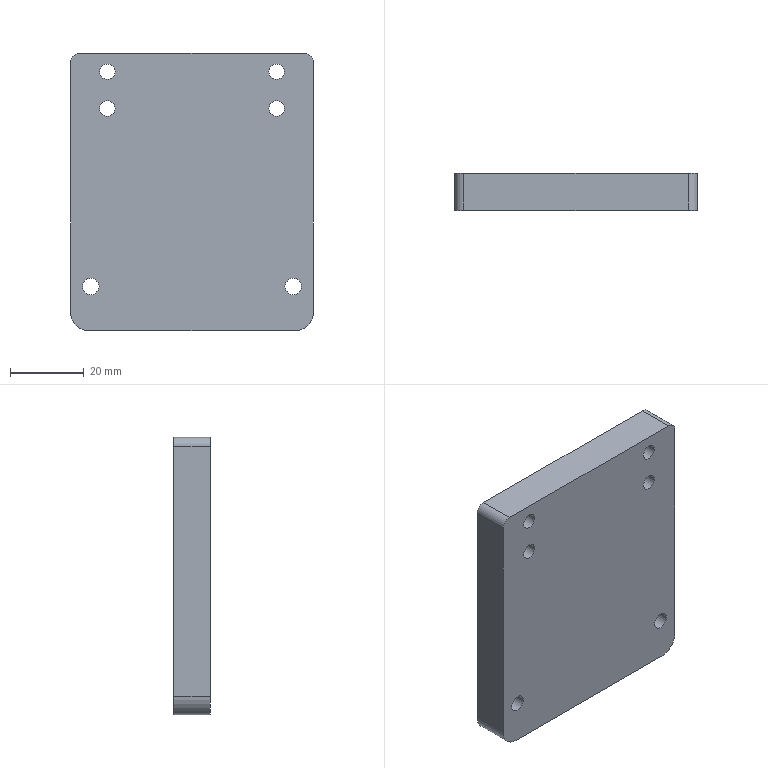Part | SolidWorks | features BaseBody 1 | 1 solid | 40 faces | box 66 x 10 x 75.35 mm | volume 47694 mm3 | cylinder 28 | plane 12 | commonest cylinder face diameters 8 x12 4.2 x8 4.5 x4 5 x2 10 x2
STEP:
#1=CARTESIAN_POINT('',(-707.631,758.297,277.132));
#2=VERTEX_POINT('',#1);
#3=CARTESIAN_POINT('',(-702.631,758.297,282.132));
#4=VERTEX_POINT('',#3);
#5=CARTESIAN_POINT('',(-707.631,758.297,282.132));
#6=DIRECTION('',(0.,-1.,0.));
#7=DIRECTION('',(0.,0.,-1.));
#8=AXIS2_PLACEMENT_3D('',#5,#6,#7);
#9=CIRCLE('',#8,5.);
#10=EDGE_CURVE('',#2,#4,#9,.T.);
#11=ORIENTED_EDGE('',*,*,#10,.F.);
#12=CARTESIAN_POINT('',(-763.631,758.297,277.132));
#13=VERTEX_POINT('',#12);
#14=CARTESIAN_POINT('',(-763.631,758.297,277.132));
#15=DIRECTION('',(1.,0.,0.));
#16=VECTOR('',#15,1000.);
#17=LINE('',#14,#16);
#18=EDGE_CURVE('',#13,#2,#17,.T.);
#19=ORIENTED_EDGE('',*,*,#18,.F.);
#20=CARTESIAN_POINT('',(-768.631,758.297,282.132));
#21=VERTEX_POINT('',#20);
#22=CARTESIAN_POINT('',(-763.631,758.297,282.132));
#23=DIRECTION('',(0.,-1.,0.));
#24=DIRECTION('',(-1.,0.,0.));
#25=AXIS2_PLACEMENT_3D('',#22,#23,#24);
#26=CIRCLE('',#25,5.);
#27=EDGE_CURVE('',#21,#13,#26,.T.);
#28=ORIENTED_EDGE('',*,*,#27,.F.);
#29=CARTESIAN_POINT('',(-768.631,758.297,349.982));
#30=VERTEX_POINT('',#29);
#31=CARTESIAN_POINT('',(-768.631,758.297,349.982));
#32=DIRECTION('',(0.,0.,-1.));
#33=VECTOR('',#32,1000.);
#34=LINE('',#31,#33);
#35=EDGE_CURVE('',#30,#21,#34,.T.);
#36=ORIENTED_EDGE('',*,*,#35,.F.);
#37=CARTESIAN_POINT('',(-766.131,758.297,352.482));
#38=VERTEX_POINT('',#37);
#39=CARTESIAN_POINT('',(-766.131,758.297,349.982));
#40=DIRECTION('',(0.,-1.,0.));
#41=DIRECTION('',(0.,0.,1.));
#42=AXIS2_PLACEMENT_3D('',#39,#40,#41);
#43=CIRCLE('',#42,2.5);
#44=EDGE_CURVE('',#38,#30,#43,.T.);
#45=ORIENTED_EDGE('',*,*,#44,.F.);
#46=CARTESIAN_POINT('',(-705.131,758.297,352.482));
#47=VERTEX_POINT('',#46);
#48=CARTESIAN_POINT('',(-705.131,758.297,352.482));
#49=DIRECTION('',(-1.,0.,0.));
#50=VECTOR('',#49,1000.);
#51=LINE('',#48,#50);
#52=EDGE_CURVE('',#47,#38,#51,.T.);
#53=ORIENTED_EDGE('',*,*,#52,.F.);
#54=CARTESIAN_POINT('',(-702.631,758.297,349.982));
#55=VERTEX_POINT('',#54);
#56=CARTESIAN_POINT('',(-705.131,758.297,349.982));
#57=DIRECTION('',(0.,-1.,0.));
#58=DIRECTION('',(1.,0.,0.));
#59=AXIS2_PLACEMENT_3D('',#56,#57,#58);
#60=CIRCLE('',#59,2.5);
#61=EDGE_CURVE('',#55,#47,#60,.T.);
#62=ORIENTED_EDGE('',*,*,#61,.F.);
#63=CARTESIAN_POINT('',(-702.631,758.297,282.132));
#64=DIRECTION('',(0.,0.,1.));
#65=VECTOR('',#64,1000.);
#66=LINE('',#63,#65);
#67=EDGE_CURVE('',#4,#55,#66,.T.);
#68=ORIENTED_EDGE('',*,*,#67,.F.);
#69=EDGE_LOOP('',(#11,#19,#28,#36,#45,#53,#62,#68));
#70=FACE_OUTER_BOUND('',#69,.T.);
#71=CARTESIAN_POINT('',(-712.131,758.297,289.132));
#72=VERTEX_POINT('',#71);
#73=CARTESIAN_POINT('',(-704.131,758.297,289.132));
#74=VERTEX_POINT('',#73);
#75=CARTESIAN_POINT('',(-708.131,758.297,289.132));
#76=DIRECTION('',(0.,1.,0.));
#77=DIRECTION('',(-1.,0.,0.));
#78=AXIS2_PLACEMENT_3D('',#75,#76,#77);
#79=CIRCLE('',#78,4.);
#80=EDGE_CURVE('',#72,#74,#79,.T.);
#81=ORIENTED_EDGE('',*,*,#80,.F.);
#82=CARTESIAN_POINT('',(-708.131,758.297,289.132));
#83=DIRECTION('',(0.,1.,0.));
#84=DIRECTION('',(1.,0.,0.));
#85=AXIS2_PLACEMENT_3D('',#82,#83,#84);
#86=CIRCLE('',#85,4.);
#87=EDGE_CURVE('',#74,#72,#86,.T.);
#88=ORIENTED_EDGE('',*,*,#87,.F.);
#89=EDGE_LOOP('',(#81,#88));
#90=FACE_BOUND('',#89,.T.);
#91=CARTESIAN_POINT('',(-716.631,758.297,347.482));
#92=VERTEX_POINT('',#91);
#93=CARTESIAN_POINT('',(-708.631,758.297,347.482));
#94=VERTEX_POINT('',#93);
#95=CARTESIAN_POINT('',(-712.631,758.297,347.482));
#96=DIRECTION('',(0.,1.,0.));
#97=DIRECTION('',(-1.,0.,0.));
#98=AXIS2_PLACEMENT_3D('',#95,#96,#97);
#99=CIRCLE('',#98,4.);
#100=EDGE_CURVE('',#92,#94,#99,.T.);
#101=ORIENTED_EDGE('',*,*,#100,.F.);
#102=CARTESIAN_POINT('',(-712.631,758.297,347.482));
#103=DIRECTION('',(0.,1.,0.));
#104=DIRECTION('',(1.,0.,0.));
#105=AXIS2_PLACEMENT_3D('',#102,#103,#104);
#106=CIRCLE('',#105,4.);
#107=EDGE_CURVE('',#94,#92,#106,.T.);
#108=ORIENTED_EDGE('',*,*,#107,.F.);
#109=EDGE_LOOP('',(#101,#108));
#110=FACE_BOUND('',#109,.T.);
#111=CARTESIAN_POINT('',(-762.631,758.297,347.482));
#112=VERTEX_POINT('',#111);
#113=CARTESIAN_POINT('',(-754.631,758.297,347.482));
#114=VERTEX_POINT('',#113);
#115=CARTESIAN_POINT('',(-758.631,758.297,347.482));
#116=DIRECTION('',(0.,1.,0.));
#117=DIRECTION('',(-1.,0.,0.));
#118=AXIS2_PLACEMENT_3D('',#115,#116,#117);
#119=CIRCLE('',#118,4.);
#120=EDGE_CURVE('',#112,#114,#119,.T.);
#121=ORIENTED_EDGE('',*,*,#120,.F.);
#122=CARTESIAN_POINT('',(-758.631,758.297,347.482));
#123=DIRECTION('',(0.,1.,0.));
#124=DIRECTION('',(1.,0.,0.));
#125=AXIS2_PLACEMENT_3D('',#122,#123,#124);
#126=CIRCLE('',#125,4.);
#127=EDGE_CURVE('',#114,#112,#126,.T.);
#128=ORIENTED_EDGE('',*,*,#127,.F.);
#129=EDGE_LOOP('',(#121,#128));
#130=FACE_BOUND('',#129,.T.);
#131=CARTESIAN_POINT('',(-762.631,758.297,337.482));
#132=VERTEX_POINT('',#131);
#133=CARTESIAN_POINT('',(-754.631,758.297,337.482));
#134=VERTEX_POINT('',#133);
#135=CARTESIAN_POINT('',(-758.631,758.297,337.482));
#136=DIRECTION('',(0.,1.,0.));
#137=DIRECTION('',(-1.,0.,0.));
#138=AXIS2_PLACEMENT_3D('',#135,#136,#137);
#139=CIRCLE('',#138,4.);
#140=EDGE_CURVE('',#132,#134,#139,.T.);
#141=ORIENTED_EDGE('',*,*,#140,.F.);
#142=CARTESIAN_POINT('',(-758.631,758.297,337.482));
#143=DIRECTION('',(0.,1.,0.));
#144=DIRECTION('',(1.,0.,0.));
#145=AXIS2_PLACEMENT_3D('',#142,#143,#144);
#146=CIRCLE('',#145,4.);
#147=EDGE_CURVE('',#134,#132,#146,.T.);
#148=ORIENTED_EDGE('',*,*,#147,.F.);
#149=EDGE_LOOP('',(#141,#148));
#150=FACE_BOUND('',#149,.T.);
#151=CARTESIAN_POINT('',(-716.631,758.297,337.482));
#152=VERTEX_POINT('',#151);
#153=CARTESIAN_POINT('',(-708.631,758.297,337.482));
#154=VERTEX_POINT('',#153);
#155=CARTESIAN_POINT('',(-712.631,758.297,337.482));
#156=DIRECTION('',(0.,1.,0.));
#157=DIRECTION('',(-1.,0.,0.));
#158=AXIS2_PLACEMENT_3D('',#155,#156,#157);
#159=CIRCLE('',#158,4.);
#160=EDGE_CURVE('',#152,#154,#159,.T.);
#161=ORIENTED_EDGE('',*,*,#160,.F.);
#162=CARTESIAN_POINT('',(-712.631,758.297,337.482));
#163=DIRECTION('',(0.,1.,0.));
#164=DIRECTION('',(1.,0.,0.));
#165=AXIS2_PLACEMENT_3D('',#162,#163,#164);
#166=CIRCLE('',#165,4.);
#167=EDGE_CURVE('',#154,#152,#166,.T.);
#168=ORIENTED_EDGE('',*,*,#167,.F.);
#169=EDGE_LOOP('',(#161,#168));
#170=FACE_BOUND('',#169,.T.);
#171=CARTESIAN_POINT('',(-767.131,758.297,289.132));
#172=VERTEX_POINT('',#171);
#173=CARTESIAN_POINT('',(-759.131,758.297,289.132));
#174=VERTEX_POINT('',#173);
#175=CARTESIAN_POINT('',(-763.131,758.297,289.132));
#176=DIRECTION('',(0.,1.,0.));
#177=DIRECTION('',(-1.,0.,0.));
#178=AXIS2_PLACEMENT_3D('',#175,#176,#177);
#179=CIRCLE('',#178,4.);
#180=EDGE_CURVE('',#172,#174,#179,.T.);
#181=ORIENTED_EDGE('',*,*,#180,.F.);
#182=CARTESIAN_POINT('',(-763.131,758.297,289.132));
#183=DIRECTION('',(0.,1.,0.));
#184=DIRECTION('',(1.,0.,0.));
#185=AXIS2_PLACEMENT_3D('',#182,#183,#184);
#186=CIRCLE('',#185,4.);
#187=EDGE_CURVE('',#174,#172,#186,.T.);
#188=ORIENTED_EDGE('',*,*,#187,.F.);
#189=EDGE_LOOP('',(#181,#188));
#190=FACE_BOUND('',#189,.T.);
#191=CARTESIAN_POINT('',(-735.631,758.297,320.932));
#192=DIRECTION('',(0.,1.,0.));
#193=DIRECTION('',(1.,0.,0.));
#194=AXIS2_PLACEMENT_3D('',#191,#192,#193);
#195=PLANE('',#194);
#196=ADVANCED_FACE('',(#70,#90,#110,#130,#150,#170,#190),#195,.T.);
#197=CARTESIAN_POINT('',(-702.631,748.297,282.132));
#198=VERTEX_POINT('',#197);
#199=CARTESIAN_POINT('',(-702.631,748.297,282.132));
#200=DIRECTION('',(0.,1.,0.));
#201=VECTOR('',#200,1000.);
#202=LINE('',#199,#201);
#203=EDGE_CURVE('',#198,#4,#202,.T.);
#204=ORIENTED_EDGE('',*,*,#203,.T.);
#205=ORIENTED_EDGE('',*,*,#67,.T.);
#206=CARTESIAN_POINT('',(-702.631,748.297,349.982));
#207=VERTEX_POINT('',#206);
#208=CARTESIAN_POINT('',(-702.631,758.297,349.982));
#209=DIRECTION('',(0.,-1.,0.));
#210=VECTOR('',#209,1000.);
#211=LINE('',#208,#210);
#212=EDGE_CURVE('',#55,#207,#211,.T.);
#213=ORIENTED_EDGE('',*,*,#212,.T.);
#214=CARTESIAN_POINT('',(-702.631,748.297,349.982));
#215=DIRECTION('',(0.,0.,-1.));
#216=VECTOR('',#215,1000.);
#217=LINE('',#214,#216);
#218=EDGE_CURVE('',#207,#198,#217,.T.);
#219=ORIENTED_EDGE('',*,*,#218,.T.);
#220=EDGE_LOOP('',(#204,#205,#213,#219));
#221=FACE_OUTER_BOUND('',#220,.T.);
#222=CARTESIAN_POINT('',(-702.631,758.297,277.132));
#223=DIRECTION('',(-1.,0.,0.));
#224=DIRECTION('',(0.,1.,0.));
#225=AXIS2_PLACEMENT_3D('',#222,#223,#224);
#226=PLANE('',#225);
#227=ADVANCED_FACE('',(#221),#226,.F.);
#228=CARTESIAN_POINT('',(-768.631,748.297,349.982));
#229=VERTEX_POINT('',#228);
#230=CARTESIAN_POINT('',(-766.131,748.297,352.482));
#231=VERTEX_POINT('',#230);
#232=CARTESIAN_POINT('',(-766.131,748.297,349.982));
#233=DIRECTION('',(0.,1.,0.));
#234=DIRECTION('',(-1.,0.,0.));
#235=AXIS2_PLACEMENT_3D('',#232,#233,#234);
#236=CIRCLE('',#235,2.5);
#237=EDGE_CURVE('',#229,#231,#236,.T.);
#238=ORIENTED_EDGE('',*,*,#237,.F.);
#239=CARTESIAN_POINT('',(-768.631,748.297,282.132));
#240=VERTEX_POINT('',#239);
#241=CARTESIAN_POINT('',(-768.631,748.297,282.132));
#242=DIRECTION('',(0.,0.,1.));
#243=VECTOR('',#242,1000.);
#244=LINE('',#241,#243);
#245=EDGE_CURVE('',#240,#229,#244,.T.);
#246=ORIENTED_EDGE('',*,*,#245,.F.);
#247=CARTESIAN_POINT('',(-763.631,748.297,277.132));
#248=VERTEX_POINT('',#247);
#249=CARTESIAN_POINT('',(-763.631,748.297,282.132));
#250=DIRECTION('',(0.,1.,0.));
#251=DIRECTION('',(0.,0.,-1.));
#252=AXIS2_PLACEMENT_3D('',#249,#250,#251);
#253=CIRCLE('',#252,5.);
#254=EDGE_CURVE('',#248,#240,#253,.T.);
#255=ORIENTED_EDGE('',*,*,#254,.F.);
#256=CARTESIAN_POINT('',(-707.631,748.297,277.132));
#257=VERTEX_POINT('',#256);
#258=CARTESIAN_POINT('',(-707.631,748.297,277.132));
#259=DIRECTION('',(-1.,0.,0.));
#260=VECTOR('',#259,1000.);
#261=LINE('',#258,#260);
#262=EDGE_CURVE('',#257,#248,#261,.T.);
#263=ORIENTED_EDGE('',*,*,#262,.F.);
#264=CARTESIAN_POINT('',(-707.631,748.297,282.132));
#265=DIRECTION('',(0.,1.,0.));
#266=DIRECTION('',(1.,0.,0.));
#267=AXIS2_PLACEMENT_3D('',#264,#265,#266);
#268=CIRCLE('',#267,5.);
#269=EDGE_CURVE('',#198,#257,#268,.T.);
#270=ORIENTED_EDGE('',*,*,#269,.F.);
#271=ORIENTED_EDGE('',*,*,#218,.F.);
#272=CARTESIAN_POINT('',(-705.131,748.297,352.482));
#273=VERTEX_POINT('',#272);
#274=CARTESIAN_POINT('',(-705.131,748.297,349.982));
#275=DIRECTION('',(0.,1.,0.));
#276=DIRECTION('',(0.,0.,1.));
#277=AXIS2_PLACEMENT_3D('',#274,#275,#276);
#278=CIRCLE('',#277,2.5);
#279=EDGE_CURVE('',#273,#207,#278,.T.);
#280=ORIENTED_EDGE('',*,*,#279,.F.);
#281=CARTESIAN_POINT('',(-766.131,748.297,352.482));
#282=DIRECTION('',(1.,0.,0.));
#283=VECTOR('',#282,1000.);
#284=LINE('',#281,#283);
#285=EDGE_CURVE('',#231,#273,#284,.T.);
#286=ORIENTED_EDGE('',*,*,#285,.F.);
#287=EDGE_LOOP('',(#238,#246,#255,#263,#270,#271,#280,#286));
#288=FACE_OUTER_BOUND('',#287,.T.);
#289=CARTESIAN_POINT('',(-705.881,748.297,289.132));
#290=VERTEX_POINT('',#289);
#291=CARTESIAN_POINT('',(-710.381,748.297,289.132));
#292=VERTEX_POINT('',#291);
#293=CARTESIAN_POINT('',(-708.131,748.297,289.132));
#294=DIRECTION('',(0.,-1.,0.));
#295=DIRECTION('',(1.,0.,0.));
#296=AXIS2_PLACEMENT_3D('',#293,#294,#295);
#297=CIRCLE('',#296,2.25);
#298=EDGE_CURVE('',#290,#292,#297,.T.);
#299=ORIENTED_EDGE('',*,*,#298,.F.);
#300=CARTESIAN_POINT('',(-708.131,748.297,289.132));
#301=DIRECTION('',(0.,-1.,0.));
#302=DIRECTION('',(-1.,0.,0.));
#303=AXIS2_PLACEMENT_3D('',#300,#301,#302);
#304=CIRCLE('',#303,2.25);
#305=EDGE_CURVE('',#292,#290,#304,.T.);
#306=ORIENTED_EDGE('',*,*,#305,.F.);
#307=EDGE_LOOP('',(#299,#306));
#308=FACE_BOUND('',#307,.T.);
#309=CARTESIAN_POINT('',(-710.531,748.297,347.482));
#310=VERTEX_POINT('',#309);
#311=CARTESIAN_POINT('',(-714.731,748.297,347.482));
#312=VERTEX_POINT('',#311);
#313=CARTESIAN_POINT('',(-712.631,748.297,347.482));
#314=DIRECTION('',(0.,-1.,0.));
#315=DIRECTION('',(1.,0.,0.));
#316=AXIS2_PLACEMENT_3D('',#313,#314,#315);
#317=CIRCLE('',#316,2.1);
#318=EDGE_CURVE('',#310,#312,#317,.T.);
#319=ORIENTED_EDGE('',*,*,#318,.F.);
#320=CARTESIAN_POINT('',(-712.631,748.297,347.482));
#321=DIRECTION('',(0.,-1.,0.));
#322=DIRECTION('',(-1.,0.,0.));
#323=AXIS2_PLACEMENT_3D('',#320,#321,#322);
#324=CIRCLE('',#323,2.1);
#325=EDGE_CURVE('',#312,#310,#324,.T.);
#326=ORIENTED_EDGE('',*,*,#325,.F.);
#327=EDGE_LOOP('',(#319,#326));
#328=FACE_BOUND('',#327,.T.);
#329=CARTESIAN_POINT('',(-756.531,748.297,347.482));
#330=VERTEX_POINT('',#329);
#331=CARTESIAN_POINT('',(-760.731,748.297,347.482));
#332=VERTEX_POINT('',#331);
#333=CARTESIAN_POINT('',(-758.631,748.297,347.482));
#334=DIRECTION('',(0.,-1.,0.));
#335=DIRECTION('',(1.,0.,0.));
#336=AXIS2_PLACEMENT_3D('',#333,#334,#335);
#337=CIRCLE('',#336,2.1);
#338=EDGE_CURVE('',#330,#332,#337,.T.);
#339=ORIENTED_EDGE('',*,*,#338,.F.);
#340=CARTESIAN_POINT('',(-758.631,748.297,347.482));
#341=DIRECTION('',(0.,-1.,0.));
#342=DIRECTION('',(-1.,0.,0.));
#343=AXIS2_PLACEMENT_3D('',#340,#341,#342);
#344=CIRCLE('',#343,2.1);
#345=EDGE_CURVE('',#332,#330,#344,.T.);
#346=ORIENTED_EDGE('',*,*,#345,.F.);
#347=EDGE_LOOP('',(#339,#346));
#348=FACE_BOUND('',#347,.T.);
#349=CARTESIAN_POINT('',(-710.531,748.297,337.482));
#350=VERTEX_POINT('',#349);
#351=CARTESIAN_POINT('',(-714.731,748.297,337.482));
#352=VERTEX_POINT('',#351);
#353=CARTESIAN_POINT('',(-712.631,748.297,337.482));
#354=DIRECTION('',(0.,-1.,0.));
#355=DIRECTION('',(1.,0.,0.));
#356=AXIS2_PLACEMENT_3D('',#353,#354,#355);
#357=CIRCLE('',#356,2.1);
#358=EDGE_CURVE('',#350,#352,#357,.T.);
#359=ORIENTED_EDGE('',*,*,#358,.F.);
#360=CARTESIAN_POINT('',(-712.631,748.297,337.482));
#361=DIRECTION('',(0.,-1.,0.));
#362=DIRECTION('',(-1.,0.,0.));
#363=AXIS2_PLACEMENT_3D('',#360,#361,#362);
#364=CIRCLE('',#363,2.1);
#365=EDGE_CURVE('',#352,#350,#364,.T.);
#366=ORIENTED_EDGE('',*,*,#365,.F.);
#367=EDGE_LOOP('',(#359,#366));
#368=FACE_BOUND('',#367,.T.);
#369=CARTESIAN_POINT('',(-756.531,748.297,337.482));
#370=VERTEX_POINT('',#369);
#371=CARTESIAN_POINT('',(-760.731,748.297,337.482));
#372=VERTEX_POINT('',#371);
#373=CARTESIAN_POINT('',(-758.631,748.297,337.482));
#374=DIRECTION('',(0.,-1.,0.));
#375=DIRECTION('',(1.,0.,0.));
#376=AXIS2_PLACEMENT_3D('',#373,#374,#375);
#377=CIRCLE('',#376,2.1);
#378=EDGE_CURVE('',#370,#372,#377,.T.);
#379=ORIENTED_EDGE('',*,*,#378,.F.);
#380=CARTESIAN_POINT('',(-758.631,748.297,337.482));
#381=DIRECTION('',(0.,-1.,0.));
#382=DIRECTION('',(-1.,0.,0.));
#383=AXIS2_PLACEMENT_3D('',#380,#381,#382);
#384=CIRCLE('',#383,2.1);
#385=EDGE_CURVE('',#372,#370,#384,.T.);
#386=ORIENTED_EDGE('',*,*,#385,.F.);
#387=EDGE_LOOP('',(#379,#386));
#388=FACE_BOUND('',#387,.T.);
#389=CARTESIAN_POINT('',(-760.881,748.297,289.132));
#390=VERTEX_POINT('',#389);
#391=CARTESIAN_POINT('',(-765.381,748.297,289.132));
#392=VERTEX_POINT('',#391);
#393=CARTESIAN_POINT('',(-763.131,748.297,289.132));
#394=DIRECTION('',(0.,-1.,0.));
#395=DIRECTION('',(1.,0.,0.));
#396=AXIS2_PLACEMENT_3D('',#393,#394,#395);
#397=CIRCLE('',#396,2.25);
#398=EDGE_CURVE('',#390,#392,#397,.T.);
#399=ORIENTED_EDGE('',*,*,#398,.F.);
#400=CARTESIAN_POINT('',(-763.131,748.297,289.132));
#401=DIRECTION('',(0.,-1.,0.));
#402=DIRECTION('',(-1.,0.,0.));
#403=AXIS2_PLACEMENT_3D('',#400,#401,#402);
#404=CIRCLE('',#403,2.25);
#405=EDGE_CURVE('',#392,#390,#404,.T.);
#406=ORIENTED_EDGE('',*,*,#405,.F.);
#407=EDGE_LOOP('',(#399,#406));
#408=FACE_BOUND('',#407,.T.);
#409=CARTESIAN_POINT('',(-735.631,748.297,320.932));
#410=DIRECTION('',(0.,1.,0.));
#411=DIRECTION('',(1.,0.,0.));
#412=AXIS2_PLACEMENT_3D('',#409,#410,#411);
#413=PLANE('',#412);
#414=ADVANCED_FACE('',(#288,#308,#328,#348,#368,#388,#408),#413,.F.);
#415=CARTESIAN_POINT('',(-766.131,758.297,352.482));
#416=DIRECTION('',(0.,-1.,0.));
#417=VECTOR('',#416,1000.);
#418=LINE('',#415,#417);
#419=EDGE_CURVE('',#38,#231,#418,.T.);
#420=ORIENTED_EDGE('',*,*,#419,.T.);
#421=ORIENTED_EDGE('',*,*,#285,.T.);
#422=CARTESIAN_POINT('',(-705.131,748.297,352.482));
#423=DIRECTION('',(0.,1.,0.));
#424=VECTOR('',#423,1000.);
#425=LINE('',#422,#424);
#426=EDGE_CURVE('',#273,#47,#425,.T.);
#427=ORIENTED_EDGE('',*,*,#426,.T.);
#428=ORIENTED_EDGE('',*,*,#52,.T.);
#429=EDGE_LOOP('',(#420,#421,#427,#428));
#430=FACE_OUTER_BOUND('',#429,.T.);
#431=CARTESIAN_POINT('',(-691.23,758.297,352.482));
#432=DIRECTION('',(0.,0.,-1.));
#433=DIRECTION('',(1.,0.,0.));
#434=AXIS2_PLACEMENT_3D('',#431,#432,#433);
#435=PLANE('',#434);
#436=ADVANCED_FACE('',(#430),#435,.F.);
#437=ORIENTED_EDGE('',*,*,#61,.T.);
#438=ORIENTED_EDGE('',*,*,#426,.F.);
#439=ORIENTED_EDGE('',*,*,#279,.T.);
#440=ORIENTED_EDGE('',*,*,#212,.F.);
#441=EDGE_LOOP('',(#437,#438,#439,#440));
#442=FACE_OUTER_BOUND('',#441,.T.);
#443=CARTESIAN_POINT('',(-705.131,771.333,349.982));
#444=DIRECTION('',(0.,-1.,0.));
#445=DIRECTION('',(-1.,0.,0.));
#446=AXIS2_PLACEMENT_3D('',#443,#444,#445);
#447=CYLINDRICAL_SURFACE('',#446,2.5);
#448=ADVANCED_FACE('',(#442),#447,.T.);
#449=ORIENTED_EDGE('',*,*,#237,.T.);
#450=ORIENTED_EDGE('',*,*,#419,.F.);
#451=ORIENTED_EDGE('',*,*,#44,.T.);
#452=CARTESIAN_POINT('',(-768.631,748.297,349.982));
#453=DIRECTION('',(0.,1.,0.));
#454=VECTOR('',#453,1000.);
#455=LINE('',#452,#454);
#456=EDGE_CURVE('',#229,#30,#455,.T.);
#457=ORIENTED_EDGE('',*,*,#456,.F.);
#458=EDGE_LOOP('',(#449,#450,#451,#457));
#459=FACE_OUTER_BOUND('',#458,.T.);
#460=CARTESIAN_POINT('',(-766.131,735.261,349.982));
#461=DIRECTION('',(0.,1.,0.));
#462=DIRECTION('',(1.,0.,0.));
#463=AXIS2_PLACEMENT_3D('',#460,#461,#462);
#464=CYLINDRICAL_SURFACE('',#463,2.5);
#465=ADVANCED_FACE('',(#459),#464,.T.);
#466=CARTESIAN_POINT('',(-768.631,758.297,282.132));
#467=DIRECTION('',(0.,-1.,0.));
#468=VECTOR('',#467,1000.);
#469=LINE('',#466,#468);
#470=EDGE_CURVE('',#21,#240,#469,.T.);
#471=ORIENTED_EDGE('',*,*,#470,.T.);
#472=ORIENTED_EDGE('',*,*,#245,.T.);
#473=ORIENTED_EDGE('',*,*,#456,.T.);
#474=ORIENTED_EDGE('',*,*,#35,.T.);
#475=EDGE_LOOP('',(#471,#472,#473,#474));
#476=FACE_OUTER_BOUND('',#475,.T.);
#477=CARTESIAN_POINT('',(-768.631,758.297,277.132));
#478=DIRECTION('',(1.,0.,0.));
#479=DIRECTION('',(0.,-1.,0.));
#480=AXIS2_PLACEMENT_3D('',#477,#478,#479);
#481=PLANE('',#480);
#482=ADVANCED_FACE('',(#476),#481,.F.);
#483=ORIENTED_EDGE('',*,*,#254,.T.);
#484=ORIENTED_EDGE('',*,*,#470,.F.);
#485=ORIENTED_EDGE('',*,*,#27,.T.);
#486=CARTESIAN_POINT('',(-763.631,748.297,277.132));
#487=DIRECTION('',(0.,1.,0.));
#488=VECTOR('',#487,1000.);
#489=LINE('',#486,#488);
#490=EDGE_CURVE('',#248,#13,#489,.T.);
#491=ORIENTED_EDGE('',*,*,#490,.F.);
#492=EDGE_LOOP('',(#483,#484,#485,#491));
#493=FACE_OUTER_BOUND('',#492,.T.);
#494=CARTESIAN_POINT('',(-763.631,758.297,282.132));
#495=DIRECTION('',(0.,-1.,0.));
#496=DIRECTION('',(-1.,0.,0.));
#497=AXIS2_PLACEMENT_3D('',#494,#495,#496);
#498=CYLINDRICAL_SURFACE('',#497,5.);
#499=ADVANCED_FACE('',(#493),#498,.T.);
#500=ORIENTED_EDGE('',*,*,#262,.T.);
#501=ORIENTED_EDGE('',*,*,#490,.T.);
#502=ORIENTED_EDGE('',*,*,#18,.T.);
#503=CARTESIAN_POINT('',(-707.631,758.297,277.132));
#504=DIRECTION('',(0.,-1.,0.));
#505=VECTOR('',#504,1000.);
#506=LINE('',#503,#505);
#507=EDGE_CURVE('',#2,#257,#506,.T.);
#508=ORIENTED_EDGE('',*,*,#507,.T.);
#509=EDGE_LOOP('',(#500,#501,#502,#508));
#510=FACE_OUTER_BOUND('',#509,.T.);
#511=CARTESIAN_POINT('',(-768.631,758.297,277.132));
#512=DIRECTION('',(0.,0.,1.));
#513=DIRECTION('',(-1.,0.,0.));
#514=AXIS2_PLACEMENT_3D('',#511,#512,#513);
#515=PLANE('',#514);
#516=ADVANCED_FACE('',(#510),#515,.F.);
#517=ORIENTED_EDGE('',*,*,#269,.T.);
#518=ORIENTED_EDGE('',*,*,#507,.F.);
#519=ORIENTED_EDGE('',*,*,#10,.T.);
#520=ORIENTED_EDGE('',*,*,#203,.F.);
#521=EDGE_LOOP('',(#517,#518,#519,#520));
#522=FACE_OUTER_BOUND('',#521,.T.);
#523=CARTESIAN_POINT('',(-707.631,758.297,282.132));
#524=DIRECTION('',(0.,-1.,0.));
#525=DIRECTION('',(-1.,0.,0.));
#526=AXIS2_PLACEMENT_3D('',#523,#524,#525);
#527=CYLINDRICAL_SURFACE('',#526,5.);
#528=ADVANCED_FACE('',(#522),#527,.T.);
#529=CARTESIAN_POINT('',(-705.881,753.897,289.132));
#530=VERTEX_POINT('',#529);
#531=CARTESIAN_POINT('',(-710.381,753.897,289.132));
#532=VERTEX_POINT('',#531);
#533=CARTESIAN_POINT('',(-708.131,753.897,289.132));
#534=DIRECTION('',(0.,1.,0.));
#535=DIRECTION('',(1.,0.,0.));
#536=AXIS2_PLACEMENT_3D('',#533,#534,#535);
#537=CIRCLE('',#536,2.25);
#538=EDGE_CURVE('',#530,#532,#537,.T.);
#539=ORIENTED_EDGE('',*,*,#538,.T.);
#540=CARTESIAN_POINT('',(-710.381,753.897,289.132));
#541=DIRECTION('',(0.,-1.,0.));
#542=VECTOR('',#541,1000.);
#543=LINE('',#540,#542);
#544=EDGE_CURVE('',#532,#292,#543,.T.);
#545=ORIENTED_EDGE('',*,*,#544,.T.);
#546=ORIENTED_EDGE('',*,*,#305,.T.);
#547=CARTESIAN_POINT('',(-705.881,748.297,289.132));
#548=DIRECTION('',(0.,1.,0.));
#549=VECTOR('',#548,1000.);
#550=LINE('',#547,#549);
#551=EDGE_CURVE('',#290,#530,#550,.T.);
#552=ORIENTED_EDGE('',*,*,#551,.T.);
#553=EDGE_LOOP('',(#539,#545,#546,#552));
#554=FACE_OUTER_BOUND('',#553,.T.);
#555=CARTESIAN_POINT('',(-708.131,758.297,289.132));
#556=DIRECTION('',(0.,1.,0.));
#557=DIRECTION('',(1.,0.,0.));
#558=AXIS2_PLACEMENT_3D('',#555,#556,#557);
#559=CYLINDRICAL_SURFACE('',#558,2.25);
#560=ADVANCED_FACE('',(#554),#559,.F.);
#561=ORIENTED_EDGE('',*,*,#544,.F.);
#562=CARTESIAN_POINT('',(-708.131,753.897,289.132));
#563=DIRECTION('',(0.,1.,0.));
#564=DIRECTION('',(-1.,0.,0.));
#565=AXIS2_PLACEMENT_3D('',#562,#563,#564);
#566=CIRCLE('',#565,2.25);
#567=EDGE_CURVE('',#532,#530,#566,.T.);
#568=ORIENTED_EDGE('',*,*,#567,.T.);
#569=ORIENTED_EDGE('',*,*,#551,.F.);
#570=ORIENTED_EDGE('',*,*,#298,.T.);
#571=EDGE_LOOP('',(#561,#568,#569,#570));
#572=FACE_OUTER_BOUND('',#571,.T.);
#573=CARTESIAN_POINT('',(-708.131,758.297,289.132));
#574=DIRECTION('',(0.,1.,0.));
#575=DIRECTION('',(1.,0.,0.));
#576=AXIS2_PLACEMENT_3D('',#573,#574,#575);
#577=CYLINDRICAL_SURFACE('',#576,2.25);
#578=ADVANCED_FACE('',(#572),#577,.F.);
#579=CARTESIAN_POINT('',(-704.131,753.897,289.132));
#580=VERTEX_POINT('',#579);
#581=CARTESIAN_POINT('',(-712.131,753.897,289.132));
#582=VERTEX_POINT('',#581);
#583=CARTESIAN_POINT('',(-708.131,753.897,289.132));
#584=DIRECTION('',(0.,-1.,0.));
#585=DIRECTION('',(1.,0.,0.));
#586=AXIS2_PLACEMENT_3D('',#583,#584,#585);
#587=CIRCLE('',#586,4.);
#588=EDGE_CURVE('',#580,#582,#587,.T.);
#589=ORIENTED_EDGE('',*,*,#588,.F.);
#590=CARTESIAN_POINT('',(-708.131,753.897,289.132));
#591=DIRECTION('',(0.,-1.,0.));
#592=DIRECTION('',(-1.,0.,0.));
#593=AXIS2_PLACEMENT_3D('',#590,#591,#592);
#594=CIRCLE('',#593,4.);
#595=EDGE_CURVE('',#582,#580,#594,.T.);
#596=ORIENTED_EDGE('',*,*,#595,.F.);
#597=EDGE_LOOP('',(#589,#596));
#598=FACE_OUTER_BOUND('',#597,.T.);
#599=ORIENTED_EDGE('',*,*,#567,.F.);
#600=ORIENTED_EDGE('',*,*,#538,.F.);
#601=EDGE_LOOP('',(#599,#600));
#602=FACE_BOUND('',#601,.T.);
#603=CARTESIAN_POINT('',(-710.381,753.897,289.132));
#604=DIRECTION('',(0.,-1.,0.));
#605=DIRECTION('',(-1.,0.,0.));
#606=AXIS2_PLACEMENT_3D('',#603,#604,#605);
#607=PLANE('',#606);
#608=ADVANCED_FACE('',(#598,#602),#607,.F.);
#609=ORIENTED_EDGE('',*,*,#87,.T.);
#610=CARTESIAN_POINT('',(-712.131,758.297,289.132));
#611=DIRECTION('',(0.,-1.,0.));
#612=VECTOR('',#611,1000.);
#613=LINE('',#610,#612);
#614=EDGE_CURVE('',#72,#582,#613,.T.);
#615=ORIENTED_EDGE('',*,*,#614,.T.);
#616=ORIENTED_EDGE('',*,*,#595,.T.);
#617=CARTESIAN_POINT('',(-704.131,753.897,289.132));
#618=DIRECTION('',(0.,1.,0.));
#619=VECTOR('',#618,1000.);
#620=LINE('',#617,#619);
#621=EDGE_CURVE('',#580,#74,#620,.T.);
#622=ORIENTED_EDGE('',*,*,#621,.T.);
#623=EDGE_LOOP('',(#609,#615,#616,#622));
#624=FACE_OUTER_BOUND('',#623,.T.);
#625=CARTESIAN_POINT('',(-708.131,758.297,289.132));
#626=DIRECTION('',(0.,1.,0.));
#627=DIRECTION('',(1.,0.,0.));
#628=AXIS2_PLACEMENT_3D('',#625,#626,#627);
#629=CYLINDRICAL_SURFACE('',#628,4.);
#630=ADVANCED_FACE('',(#624),#629,.F.);
#631=ORIENTED_EDGE('',*,*,#614,.F.);
#632=ORIENTED_EDGE('',*,*,#80,.T.);
#633=ORIENTED_EDGE('',*,*,#621,.F.);
#634=ORIENTED_EDGE('',*,*,#588,.T.);
#635=EDGE_LOOP('',(#631,#632,#633,#634));
#636=FACE_OUTER_BOUND('',#635,.T.);
#637=CARTESIAN_POINT('',(-708.131,758.297,289.132));
#638=DIRECTION('',(0.,1.,0.));
#639=DIRECTION('',(1.,0.,0.));
#640=AXIS2_PLACEMENT_3D('',#637,#638,#639);
#641=CYLINDRICAL_SURFACE('',#640,4.);
#642=ADVANCED_FACE('',(#636),#641,.F.);
#643=ORIENTED_EDGE('',*,*,#325,.T.);
#644=CARTESIAN_POINT('',(-710.531,753.297,347.482));
#645=VERTEX_POINT('',#644);
#646=CARTESIAN_POINT('',(-710.531,748.297,347.482));
#647=DIRECTION('',(0.,1.,0.));
#648=VECTOR('',#647,1000.);
#649=LINE('',#646,#648);
#650=EDGE_CURVE('',#310,#645,#649,.T.);
#651=ORIENTED_EDGE('',*,*,#650,.T.);
#652=CARTESIAN_POINT('',(-714.731,753.297,347.482));
#653=VERTEX_POINT('',#652);
#654=CARTESIAN_POINT('',(-712.631,753.297,347.482));
#655=DIRECTION('',(0.,1.,0.));
#656=DIRECTION('',(1.,0.,0.));
#657=AXIS2_PLACEMENT_3D('',#654,#655,#656);
#658=CIRCLE('',#657,2.1);
#659=EDGE_CURVE('',#645,#653,#658,.T.);
#660=ORIENTED_EDGE('',*,*,#659,.T.);
#661=CARTESIAN_POINT('',(-714.731,753.297,347.482));
#662=DIRECTION('',(0.,-1.,0.));
#663=VECTOR('',#662,1000.);
#664=LINE('',#661,#663);
#665=EDGE_CURVE('',#653,#312,#664,.T.);
#666=ORIENTED_EDGE('',*,*,#665,.T.);
#667=EDGE_LOOP('',(#643,#651,#660,#666));
#668=FACE_OUTER_BOUND('',#667,.T.);
#669=CARTESIAN_POINT('',(-712.631,758.297,347.482));
#670=DIRECTION('',(0.,1.,0.));
#671=DIRECTION('',(1.,0.,0.));
#672=AXIS2_PLACEMENT_3D('',#669,#670,#671);
#673=CYLINDRICAL_SURFACE('',#672,2.1);
#674=ADVANCED_FACE('',(#668),#673,.F.);
#675=ORIENTED_EDGE('',*,*,#318,.T.);
#676=ORIENTED_EDGE('',*,*,#665,.F.);
#677=CARTESIAN_POINT('',(-712.631,753.297,347.482));
#678=DIRECTION('',(0.,1.,0.));
#679=DIRECTION('',(-1.,0.,0.));
#680=AXIS2_PLACEMENT_3D('',#677,#678,#679);
#681=CIRCLE('',#680,2.1);
#682=EDGE_CURVE('',#653,#645,#681,.T.);
#683=ORIENTED_EDGE('',*,*,#682,.T.);
#684=ORIENTED_EDGE('',*,*,#650,.F.);
#685=EDGE_LOOP('',(#675,#676,#683,#684));
#686=FACE_OUTER_BOUND('',#685,.T.);
#687=CARTESIAN_POINT('',(-712.631,758.297,347.482));
#688=DIRECTION('',(0.,1.,0.));
#689=DIRECTION('',(1.,0.,0.));
#690=AXIS2_PLACEMENT_3D('',#687,#688,#689);
#691=CYLINDRICAL_SURFACE('',#690,2.1);
#692=ADVANCED_FACE('',(#686),#691,.F.);
#693=CARTESIAN_POINT('',(-708.631,753.297,347.482));
#694=VERTEX_POINT('',#693);
#695=CARTESIAN_POINT('',(-716.631,753.297,347.482));
#696=VERTEX_POINT('',#695);
#697=CARTESIAN_POINT('',(-712.631,753.297,347.482));
#698=DIRECTION('',(0.,-1.,0.));
#699=DIRECTION('',(1.,0.,0.));
#700=AXIS2_PLACEMENT_3D('',#697,#698,#699);
#701=CIRCLE('',#700,4.);
#702=EDGE_CURVE('',#694,#696,#701,.T.);
#703=ORIENTED_EDGE('',*,*,#702,.F.);
#704=CARTESIAN_POINT('',(-712.631,753.297,347.482));
#705=DIRECTION('',(0.,-1.,0.));
#706=DIRECTION('',(-1.,0.,0.));
#707=AXIS2_PLACEMENT_3D('',#704,#705,#706);
#708=CIRCLE('',#707,4.);
#709=EDGE_CURVE('',#696,#694,#708,.T.);
#710=ORIENTED_EDGE('',*,*,#709,.F.);
#711=EDGE_LOOP('',(#703,#710));
#712=FACE_OUTER_BOUND('',#711,.T.);
#713=ORIENTED_EDGE('',*,*,#682,.F.);
#714=ORIENTED_EDGE('',*,*,#659,.F.);
#715=EDGE_LOOP('',(#713,#714));
#716=FACE_BOUND('',#715,.T.);
#717=CARTESIAN_POINT('',(-735.631,753.297,320.932));
#718=DIRECTION('',(0.,1.,0.));
#719=DIRECTION('',(1.,0.,0.));
#720=AXIS2_PLACEMENT_3D('',#717,#718,#719);
#721=PLANE('',#720);
#722=ADVANCED_FACE('',(#712,#716),#721,.T.);
#723=ORIENTED_EDGE('',*,*,#709,.T.);
#724=CARTESIAN_POINT('',(-708.631,753.297,347.482));
#725=DIRECTION('',(0.,1.,0.));
#726=VECTOR('',#725,1000.);
#727=LINE('',#724,#726);
#728=EDGE_CURVE('',#694,#94,#727,.T.);
#729=ORIENTED_EDGE('',*,*,#728,.T.);
#730=ORIENTED_EDGE('',*,*,#107,.T.);
#731=CARTESIAN_POINT('',(-716.631,758.297,347.482));
#732=DIRECTION('',(0.,-1.,0.));
#733=VECTOR('',#732,1000.);
#734=LINE('',#731,#733);
#735=EDGE_CURVE('',#92,#696,#734,.T.);
#736=ORIENTED_EDGE('',*,*,#735,.T.);
#737=EDGE_LOOP('',(#723,#729,#730,#736));
#738=FACE_OUTER_BOUND('',#737,.T.);
#739=CARTESIAN_POINT('',(-712.631,758.297,347.482));
#740=DIRECTION('',(0.,1.,0.));
#741=DIRECTION('',(1.,0.,0.));
#742=AXIS2_PLACEMENT_3D('',#739,#740,#741);
#743=CYLINDRICAL_SURFACE('',#742,4.);
#744=ADVANCED_FACE('',(#738),#743,.F.);
#745=ORIENTED_EDGE('',*,*,#702,.T.);
#746=ORIENTED_EDGE('',*,*,#735,.F.);
#747=ORIENTED_EDGE('',*,*,#100,.T.);
#748=ORIENTED_EDGE('',*,*,#728,.F.);
#749=EDGE_LOOP('',(#745,#746,#747,#748));
#750=FACE_OUTER_BOUND('',#749,.T.);
#751=CARTESIAN_POINT('',(-712.631,758.297,347.482));
#752=DIRECTION('',(0.,1.,0.));
#753=DIRECTION('',(1.,0.,0.));
#754=AXIS2_PLACEMENT_3D('',#751,#752,#753);
#755=CYLINDRICAL_SURFACE('',#754,4.);
#756=ADVANCED_FACE('',(#750),#755,.F.);
#757=ORIENTED_EDGE('',*,*,#345,.T.);
#758=CARTESIAN_POINT('',(-756.531,753.297,347.482));
#759=VERTEX_POINT('',#758);
#760=CARTESIAN_POINT('',(-756.531,748.297,347.482));
#761=DIRECTION('',(0.,1.,0.));
#762=VECTOR('',#761,1000.);
#763=LINE('',#760,#762);
#764=EDGE_CURVE('',#330,#759,#763,.T.);
#765=ORIENTED_EDGE('',*,*,#764,.T.);
#766=CARTESIAN_POINT('',(-760.731,753.297,347.482));
#767=VERTEX_POINT('',#766);
#768=CARTESIAN_POINT('',(-758.631,753.297,347.482));
#769=DIRECTION('',(0.,1.,0.));
#770=DIRECTION('',(1.,0.,0.));
#771=AXIS2_PLACEMENT_3D('',#768,#769,#770);
#772=CIRCLE('',#771,2.1);
#773=EDGE_CURVE('',#759,#767,#772,.T.);
#774=ORIENTED_EDGE('',*,*,#773,.T.);
#775=CARTESIAN_POINT('',(-760.731,753.297,347.482));
#776=DIRECTION('',(0.,-1.,0.));
#777=VECTOR('',#776,1000.);
#778=LINE('',#775,#777);
#779=EDGE_CURVE('',#767,#332,#778,.T.);
#780=ORIENTED_EDGE('',*,*,#779,.T.);
#781=EDGE_LOOP('',(#757,#765,#774,#780));
#782=FACE_OUTER_BOUND('',#781,.T.);
#783=CARTESIAN_POINT('',(-758.631,758.297,347.482));
#784=DIRECTION('',(0.,1.,0.));
#785=DIRECTION('',(1.,0.,0.));
#786=AXIS2_PLACEMENT_3D('',#783,#784,#785);
#787=CYLINDRICAL_SURFACE('',#786,2.1);
#788=ADVANCED_FACE('',(#782),#787,.F.);
#789=ORIENTED_EDGE('',*,*,#338,.T.);
#790=ORIENTED_EDGE('',*,*,#779,.F.);
#791=CARTESIAN_POINT('',(-758.631,753.297,347.482));
#792=DIRECTION('',(0.,1.,0.));
#793=DIRECTION('',(-1.,0.,0.));
#794=AXIS2_PLACEMENT_3D('',#791,#792,#793);
#795=CIRCLE('',#794,2.1);
#796=EDGE_CURVE('',#767,#759,#795,.T.);
#797=ORIENTED_EDGE('',*,*,#796,.T.);
#798=ORIENTED_EDGE('',*,*,#764,.F.);
#799=EDGE_LOOP('',(#789,#790,#797,#798));
#800=FACE_OUTER_BOUND('',#799,.T.);
#801=CARTESIAN_POINT('',(-758.631,758.297,347.482));
#802=DIRECTION('',(0.,1.,0.));
#803=DIRECTION('',(1.,0.,0.));
#804=AXIS2_PLACEMENT_3D('',#801,#802,#803);
#805=CYLINDRICAL_SURFACE('',#804,2.1);
#806=ADVANCED_FACE('',(#800),#805,.F.);
#807=CARTESIAN_POINT('',(-754.631,753.297,347.482));
#808=VERTEX_POINT('',#807);
#809=CARTESIAN_POINT('',(-762.631,753.297,347.482));
#810=VERTEX_POINT('',#809);
#811=CARTESIAN_POINT('',(-758.631,753.297,347.482));
#812=DIRECTION('',(0.,-1.,0.));
#813=DIRECTION('',(1.,0.,0.));
#814=AXIS2_PLACEMENT_3D('',#811,#812,#813);
#815=CIRCLE('',#814,4.);
#816=EDGE_CURVE('',#808,#810,#815,.T.);
#817=ORIENTED_EDGE('',*,*,#816,.F.);
#818=CARTESIAN_POINT('',(-758.631,753.297,347.482));
#819=DIRECTION('',(0.,-1.,0.));
#820=DIRECTION('',(-1.,0.,0.));
#821=AXIS2_PLACEMENT_3D('',#818,#819,#820);
#822=CIRCLE('',#821,4.);
#823=EDGE_CURVE('',#810,#808,#822,.T.);
#824=ORIENTED_EDGE('',*,*,#823,.F.);
#825=EDGE_LOOP('',(#817,#824));
#826=FACE_OUTER_BOUND('',#825,.T.);
#827=ORIENTED_EDGE('',*,*,#796,.F.);
#828=ORIENTED_EDGE('',*,*,#773,.F.);
#829=EDGE_LOOP('',(#827,#828));
#830=FACE_BOUND('',#829,.T.);
#831=CARTESIAN_POINT('',(-735.631,753.297,320.932));
#832=DIRECTION('',(0.,1.,0.));
#833=DIRECTION('',(1.,0.,0.));
#834=AXIS2_PLACEMENT_3D('',#831,#832,#833);
#835=PLANE('',#834);
#836=ADVANCED_FACE('',(#826,#830),#835,.T.);
#837=ORIENTED_EDGE('',*,*,#823,.T.);
#838=CARTESIAN_POINT('',(-754.631,753.297,347.482));
#839=DIRECTION('',(0.,1.,0.));
#840=VECTOR('',#839,1000.);
#841=LINE('',#838,#840);
#842=EDGE_CURVE('',#808,#114,#841,.T.);
#843=ORIENTED_EDGE('',*,*,#842,.T.);
#844=ORIENTED_EDGE('',*,*,#127,.T.);
#845=CARTESIAN_POINT('',(-762.631,758.297,347.482));
#846=DIRECTION('',(0.,-1.,0.));
#847=VECTOR('',#846,1000.);
#848=LINE('',#845,#847);
#849=EDGE_CURVE('',#112,#810,#848,.T.);
#850=ORIENTED_EDGE('',*,*,#849,.T.);
#851=EDGE_LOOP('',(#837,#843,#844,#850));
#852=FACE_OUTER_BOUND('',#851,.T.);
#853=CARTESIAN_POINT('',(-758.631,758.297,347.482));
#854=DIRECTION('',(0.,1.,0.));
#855=DIRECTION('',(1.,0.,0.));
#856=AXIS2_PLACEMENT_3D('',#853,#854,#855);
#857=CYLINDRICAL_SURFACE('',#856,4.);
#858=ADVANCED_FACE('',(#852),#857,.F.);
#859=ORIENTED_EDGE('',*,*,#816,.T.);
#860=ORIENTED_EDGE('',*,*,#849,.F.);
#861=ORIENTED_EDGE('',*,*,#120,.T.);
#862=ORIENTED_EDGE('',*,*,#842,.F.);
#863=EDGE_LOOP('',(#859,#860,#861,#862));
#864=FACE_OUTER_BOUND('',#863,.T.);
#865=CARTESIAN_POINT('',(-758.631,758.297,347.482));
#866=DIRECTION('',(0.,1.,0.));
#867=DIRECTION('',(1.,0.,0.));
#868=AXIS2_PLACEMENT_3D('',#865,#866,#867);
#869=CYLINDRICAL_SURFACE('',#868,4.);
#870=ADVANCED_FACE('',(#864),#869,.F.);
#871=ORIENTED_EDGE('',*,*,#365,.T.);
#872=CARTESIAN_POINT('',(-710.531,753.297,337.482));
#873=VERTEX_POINT('',#872);
#874=CARTESIAN_POINT('',(-710.531,748.297,337.482));
#875=DIRECTION('',(0.,1.,0.));
#876=VECTOR('',#875,1000.);
#877=LINE('',#874,#876);
#878=EDGE_CURVE('',#350,#873,#877,.T.);
#879=ORIENTED_EDGE('',*,*,#878,.T.);
#880=CARTESIAN_POINT('',(-714.731,753.297,337.482));
#881=VERTEX_POINT('',#880);
#882=CARTESIAN_POINT('',(-712.631,753.297,337.482));
#883=DIRECTION('',(0.,1.,0.));
#884=DIRECTION('',(1.,0.,0.));
#885=AXIS2_PLACEMENT_3D('',#882,#883,#884);
#886=CIRCLE('',#885,2.1);
#887=EDGE_CURVE('',#873,#881,#886,.T.);
#888=ORIENTED_EDGE('',*,*,#887,.T.);
#889=CARTESIAN_POINT('',(-714.731,753.297,337.482));
#890=DIRECTION('',(0.,-1.,0.));
#891=VECTOR('',#890,1000.);
#892=LINE('',#889,#891);
#893=EDGE_CURVE('',#881,#352,#892,.T.);
#894=ORIENTED_EDGE('',*,*,#893,.T.);
#895=EDGE_LOOP('',(#871,#879,#888,#894));
#896=FACE_OUTER_BOUND('',#895,.T.);
#897=CARTESIAN_POINT('',(-712.631,758.297,337.482));
#898=DIRECTION('',(0.,1.,0.));
#899=DIRECTION('',(1.,0.,0.));
#900=AXIS2_PLACEMENT_3D('',#897,#898,#899);
#901=CYLINDRICAL_SURFACE('',#900,2.1);
#902=ADVANCED_FACE('',(#896),#901,.F.);
#903=ORIENTED_EDGE('',*,*,#358,.T.);
#904=ORIENTED_EDGE('',*,*,#893,.F.);
#905=CARTESIAN_POINT('',(-712.631,753.297,337.482));
#906=DIRECTION('',(0.,1.,0.));
#907=DIRECTION('',(-1.,0.,0.));
#908=AXIS2_PLACEMENT_3D('',#905,#906,#907);
#909=CIRCLE('',#908,2.1);
#910=EDGE_CURVE('',#881,#873,#909,.T.);
#911=ORIENTED_EDGE('',*,*,#910,.T.);
#912=ORIENTED_EDGE('',*,*,#878,.F.);
#913=EDGE_LOOP('',(#903,#904,#911,#912));
#914=FACE_OUTER_BOUND('',#913,.T.);
#915=CARTESIAN_POINT('',(-712.631,758.297,337.482));
#916=DIRECTION('',(0.,1.,0.));
#917=DIRECTION('',(1.,0.,0.));
#918=AXIS2_PLACEMENT_3D('',#915,#916,#917);
#919=CYLINDRICAL_SURFACE('',#918,2.1);
#920=ADVANCED_FACE('',(#914),#919,.F.);
#921=CARTESIAN_POINT('',(-708.631,753.297,337.482));
#922=VERTEX_POINT('',#921);
#923=CARTESIAN_POINT('',(-716.631,753.297,337.482));
#924=VERTEX_POINT('',#923);
#925=CARTESIAN_POINT('',(-712.631,753.297,337.482));
#926=DIRECTION('',(0.,-1.,0.));
#927=DIRECTION('',(1.,0.,0.));
#928=AXIS2_PLACEMENT_3D('',#925,#926,#927);
#929=CIRCLE('',#928,4.);
#930=EDGE_CURVE('',#922,#924,#929,.T.);
#931=ORIENTED_EDGE('',*,*,#930,.F.);
#932=CARTESIAN_POINT('',(-712.631,753.297,337.482));
#933=DIRECTION('',(0.,-1.,0.));
#934=DIRECTION('',(-1.,0.,0.));
#935=AXIS2_PLACEMENT_3D('',#932,#933,#934);
#936=CIRCLE('',#935,4.);
#937=EDGE_CURVE('',#924,#922,#936,.T.);
#938=ORIENTED_EDGE('',*,*,#937,.F.);
#939=EDGE_LOOP('',(#931,#938));
#940=FACE_OUTER_BOUND('',#939,.T.);
#941=ORIENTED_EDGE('',*,*,#910,.F.);
#942=ORIENTED_EDGE('',*,*,#887,.F.);
#943=EDGE_LOOP('',(#941,#942));
#944=FACE_BOUND('',#943,.T.);
#945=CARTESIAN_POINT('',(-735.631,753.297,320.932));
#946=DIRECTION('',(0.,1.,0.));
#947=DIRECTION('',(1.,0.,0.));
#948=AXIS2_PLACEMENT_3D('',#945,#946,#947);
#949=PLANE('',#948);
#950=ADVANCED_FACE('',(#940,#944),#949,.T.);
#951=ORIENTED_EDGE('',*,*,#937,.T.);
#952=CARTESIAN_POINT('',(-708.631,753.297,337.482));
#953=DIRECTION('',(0.,1.,0.));
#954=VECTOR('',#953,1000.);
#955=LINE('',#952,#954);
#956=EDGE_CURVE('',#922,#154,#955,.T.);
#957=ORIENTED_EDGE('',*,*,#956,.T.);
#958=ORIENTED_EDGE('',*,*,#167,.T.);
#959=CARTESIAN_POINT('',(-716.631,758.297,337.482));
#960=DIRECTION('',(0.,-1.,0.));
#961=VECTOR('',#960,1000.);
#962=LINE('',#959,#961);
#963=EDGE_CURVE('',#152,#924,#962,.T.);
#964=ORIENTED_EDGE('',*,*,#963,.T.);
#965=EDGE_LOOP('',(#951,#957,#958,#964));
#966=FACE_OUTER_BOUND('',#965,.T.);
#967=CARTESIAN_POINT('',(-712.631,758.297,337.482));
#968=DIRECTION('',(0.,1.,0.));
#969=DIRECTION('',(1.,0.,0.));
#970=AXIS2_PLACEMENT_3D('',#967,#968,#969);
#971=CYLINDRICAL_SURFACE('',#970,4.);
#972=ADVANCED_FACE('',(#966),#971,.F.);
#973=ORIENTED_EDGE('',*,*,#930,.T.);
#974=ORIENTED_EDGE('',*,*,#963,.F.);
#975=ORIENTED_EDGE('',*,*,#160,.T.);
#976=ORIENTED_EDGE('',*,*,#956,.F.);
#977=EDGE_LOOP('',(#973,#974,#975,#976));
#978=FACE_OUTER_BOUND('',#977,.T.);
#979=CARTESIAN_POINT('',(-712.631,758.297,337.482));
#980=DIRECTION('',(0.,1.,0.));
#981=DIRECTION('',(1.,0.,0.));
#982=AXIS2_PLACEMENT_3D('',#979,#980,#981);
#983=CYLINDRICAL_SURFACE('',#982,4.);
#984=ADVANCED_FACE('',(#978),#983,.F.);
#985=ORIENTED_EDGE('',*,*,#385,.T.);
#986=CARTESIAN_POINT('',(-756.531,753.297,337.482));
#987=VERTEX_POINT('',#986);
#988=CARTESIAN_POINT('',(-756.531,748.297,337.482));
#989=DIRECTION('',(0.,1.,0.));
#990=VECTOR('',#989,1000.);
#991=LINE('',#988,#990);
#992=EDGE_CURVE('',#370,#987,#991,.T.);
#993=ORIENTED_EDGE('',*,*,#992,.T.);
#994=CARTESIAN_POINT('',(-760.731,753.297,337.482));
#995=VERTEX_POINT('',#994);
#996=CARTESIAN_POINT('',(-758.631,753.297,337.482));
#997=DIRECTION('',(0.,1.,0.));
#998=DIRECTION('',(1.,0.,0.));
#999=AXIS2_PLACEMENT_3D('',#996,#997,#998);
#1000=CIRCLE('',#999,2.1);
#1001=EDGE_CURVE('',#987,#995,#1000,.T.);
#1002=ORIENTED_EDGE('',*,*,#1001,.T.);
#1003=CARTESIAN_POINT('',(-760.731,753.297,337.482));
#1004=DIRECTION('',(0.,-1.,0.));
#1005=VECTOR('',#1004,1000.);
#1006=LINE('',#1003,#1005);
#1007=EDGE_CURVE('',#995,#372,#1006,.T.);
#1008=ORIENTED_EDGE('',*,*,#1007,.T.);
#1009=EDGE_LOOP('',(#985,#993,#1002,#1008));
#1010=FACE_OUTER_BOUND('',#1009,.T.);
#1011=CARTESIAN_POINT('',(-758.631,758.297,337.482));
#1012=DIRECTION('',(0.,1.,0.));
#1013=DIRECTION('',(1.,0.,0.));
#1014=AXIS2_PLACEMENT_3D('',#1011,#1012,#1013);
#1015=CYLINDRICAL_SURFACE('',#1014,2.1);
#1016=ADVANCED_FACE('',(#1010),#1015,.F.);
#1017=ORIENTED_EDGE('',*,*,#378,.T.);
#1018=ORIENTED_EDGE('',*,*,#1007,.F.);
#1019=CARTESIAN_POINT('',(-758.631,753.297,337.482));
#1020=DIRECTION('',(0.,1.,0.));
#1021=DIRECTION('',(-1.,0.,0.));
#1022=AXIS2_PLACEMENT_3D('',#1019,#1020,#1021);
#1023=CIRCLE('',#1022,2.1);
#1024=EDGE_CURVE('',#995,#987,#1023,.T.);
#1025=ORIENTED_EDGE('',*,*,#1024,.T.);
#1026=ORIENTED_EDGE('',*,*,#992,.F.);
#1027=EDGE_LOOP('',(#1017,#1018,#1025,#1026));
#1028=FACE_OUTER_BOUND('',#1027,.T.);
#1029=CARTESIAN_POINT('',(-758.631,758.297,337.482));
#1030=DIRECTION('',(0.,1.,0.));
#1031=DIRECTION('',(1.,0.,0.));
#1032=AXIS2_PLACEMENT_3D('',#1029,#1030,#1031);
#1033=CYLINDRICAL_SURFACE('',#1032,2.1);
#1034=ADVANCED_FACE('',(#1028),#1033,.F.);
#1035=CARTESIAN_POINT('',(-754.631,753.297,337.482));
#1036=VERTEX_POINT('',#1035);
#1037=CARTESIAN_POINT('',(-762.631,753.297,337.482));
#1038=VERTEX_POINT('',#1037);
#1039=CARTESIAN_POINT('',(-758.631,753.297,337.482));
#1040=DIRECTION('',(0.,-1.,0.));
#1041=DIRECTION('',(1.,0.,0.));
#1042=AXIS2_PLACEMENT_3D('',#1039,#1040,#1041);
#1043=CIRCLE('',#1042,4.);
#1044=EDGE_CURVE('',#1036,#1038,#1043,.T.);
#1045=ORIENTED_EDGE('',*,*,#1044,.F.);
#1046=CARTESIAN_POINT('',(-758.631,753.297,337.482));
#1047=DIRECTION('',(0.,-1.,0.));
#1048=DIRECTION('',(-1.,0.,0.));
#1049=AXIS2_PLACEMENT_3D('',#1046,#1047,#1048);
#1050=CIRCLE('',#1049,4.);
#1051=EDGE_CURVE('',#1038,#1036,#1050,.T.);
#1052=ORIENTED_EDGE('',*,*,#1051,.F.);
#1053=EDGE_LOOP('',(#1045,#1052));
#1054=FACE_OUTER_BOUND('',#1053,.T.);
#1055=ORIENTED_EDGE('',*,*,#1024,.F.);
#1056=ORIENTED_EDGE('',*,*,#1001,.F.);
#1057=EDGE_LOOP('',(#1055,#1056));
#1058=FACE_BOUND('',#1057,.T.);
#1059=CARTESIAN_POINT('',(-735.631,753.297,320.932));
#1060=DIRECTION('',(0.,1.,0.));
#1061=DIRECTION('',(1.,0.,0.));
#1062=AXIS2_PLACEMENT_3D('',#1059,#1060,#1061);
#1063=PLANE('',#1062);
#1064=ADVANCED_FACE('',(#1054,#1058),#1063,.T.);
#1065=ORIENTED_EDGE('',*,*,#1051,.T.);
#1066=CARTESIAN_POINT('',(-754.631,753.297,337.482));
#1067=DIRECTION('',(0.,1.,0.));
#1068=VECTOR('',#1067,1000.);
#1069=LINE('',#1066,#1068);
#1070=EDGE_CURVE('',#1036,#134,#1069,.T.);
#1071=ORIENTED_EDGE('',*,*,#1070,.T.);
#1072=ORIENTED_EDGE('',*,*,#147,.T.);
#1073=CARTESIAN_POINT('',(-762.631,758.297,337.482));
#1074=DIRECTION('',(0.,-1.,0.));
#1075=VECTOR('',#1074,1000.);
#1076=LINE('',#1073,#1075);
#1077=EDGE_CURVE('',#132,#1038,#1076,.T.);
#1078=ORIENTED_EDGE('',*,*,#1077,.T.);
#1079=EDGE_LOOP('',(#1065,#1071,#1072,#1078));
#1080=FACE_OUTER_BOUND('',#1079,.T.);
#1081=CARTESIAN_POINT('',(-758.631,758.297,337.482));
#1082=DIRECTION('',(0.,1.,0.));
#1083=DIRECTION('',(1.,0.,0.));
#1084=AXIS2_PLACEMENT_3D('',#1081,#1082,#1083);
#1085=CYLINDRICAL_SURFACE('',#1084,4.);
#1086=ADVANCED_FACE('',(#1080),#1085,.F.);
#1087=ORIENTED_EDGE('',*,*,#1044,.T.);
#1088=ORIENTED_EDGE('',*,*,#1077,.F.);
#1089=ORIENTED_EDGE('',*,*,#140,.T.);
#1090=ORIENTED_EDGE('',*,*,#1070,.F.);
#1091=EDGE_LOOP('',(#1087,#1088,#1089,#1090));
#1092=FACE_OUTER_BOUND('',#1091,.T.);
#1093=CARTESIAN_POINT('',(-758.631,758.297,337.482));
#1094=DIRECTION('',(0.,1.,0.));
#1095=DIRECTION('',(1.,0.,0.));
#1096=AXIS2_PLACEMENT_3D('',#1093,#1094,#1095);
#1097=CYLINDRICAL_SURFACE('',#1096,4.);
#1098=ADVANCED_FACE('',(#1092),#1097,.F.);
#1099=CARTESIAN_POINT('',(-760.881,753.897,289.132));
#1100=VERTEX_POINT('',#1099);
#1101=CARTESIAN_POINT('',(-765.381,753.897,289.132));
#1102=VERTEX_POINT('',#1101);
#1103=CARTESIAN_POINT('',(-763.131,753.897,289.132));
#1104=DIRECTION('',(0.,1.,0.));
#1105=DIRECTION('',(1.,0.,0.));
#1106=AXIS2_PLACEMENT_3D('',#1103,#1104,#1105);
#1107=CIRCLE('',#1106,2.25);
#1108=EDGE_CURVE('',#1100,#1102,#1107,.T.);
#1109=ORIENTED_EDGE('',*,*,#1108,.T.);
#1110=CARTESIAN_POINT('',(-765.381,753.897,289.132));
#1111=DIRECTION('',(0.,-1.,0.));
#1112=VECTOR('',#1111,1000.);
#1113=LINE('',#1110,#1112);
#1114=EDGE_CURVE('',#1102,#392,#1113,.T.);
#1115=ORIENTED_EDGE('',*,*,#1114,.T.);
#1116=ORIENTED_EDGE('',*,*,#405,.T.);
#1117=CARTESIAN_POINT('',(-760.881,748.297,289.132));
#1118=DIRECTION('',(0.,1.,0.));
#1119=VECTOR('',#1118,1000.);
#1120=LINE('',#1117,#1119);
#1121=EDGE_CURVE('',#390,#1100,#1120,.T.);
#1122=ORIENTED_EDGE('',*,*,#1121,.T.);
#1123=EDGE_LOOP('',(#1109,#1115,#1116,#1122));
#1124=FACE_OUTER_BOUND('',#1123,.T.);
#1125=CARTESIAN_POINT('',(-763.131,758.297,289.132));
#1126=DIRECTION('',(0.,1.,0.));
#1127=DIRECTION('',(1.,0.,0.));
#1128=AXIS2_PLACEMENT_3D('',#1125,#1126,#1127);
#1129=CYLINDRICAL_SURFACE('',#1128,2.25);
#1130=ADVANCED_FACE('',(#1124),#1129,.F.);
#1131=ORIENTED_EDGE('',*,*,#1114,.F.);
#1132=CARTESIAN_POINT('',(-763.131,753.897,289.132));
#1133=DIRECTION('',(0.,1.,0.));
#1134=DIRECTION('',(-1.,0.,0.));
#1135=AXIS2_PLACEMENT_3D('',#1132,#1133,#1134);
#1136=CIRCLE('',#1135,2.25);
#1137=EDGE_CURVE('',#1102,#1100,#1136,.T.);
#1138=ORIENTED_EDGE('',*,*,#1137,.T.);
#1139=ORIENTED_EDGE('',*,*,#1121,.F.);
#1140=ORIENTED_EDGE('',*,*,#398,.T.);
#1141=EDGE_LOOP('',(#1131,#1138,#1139,#1140));
#1142=FACE_OUTER_BOUND('',#1141,.T.);
#1143=CARTESIAN_POINT('',(-763.131,758.297,289.132));
#1144=DIRECTION('',(0.,1.,0.));
#1145=DIRECTION('',(1.,0.,0.));
#1146=AXIS2_PLACEMENT_3D('',#1143,#1144,#1145);
#1147=CYLINDRICAL_SURFACE('',#1146,2.25);
#1148=ADVANCED_FACE('',(#1142),#1147,.F.);
#1149=CARTESIAN_POINT('',(-759.131,753.897,289.132));
#1150=VERTEX_POINT('',#1149);
#1151=CARTESIAN_POINT('',(-767.131,753.897,289.132));
#1152=VERTEX_POINT('',#1151);
#1153=CARTESIAN_POINT('',(-763.131,753.897,289.132));
#1154=DIRECTION('',(0.,-1.,0.));
#1155=DIRECTION('',(1.,0.,0.));
#1156=AXIS2_PLACEMENT_3D('',#1153,#1154,#1155);
#1157=CIRCLE('',#1156,4.);
#1158=EDGE_CURVE('',#1150,#1152,#1157,.T.);
#1159=ORIENTED_EDGE('',*,*,#1158,.F.);
#1160=CARTESIAN_POINT('',(-763.131,753.897,289.132));
#1161=DIRECTION('',(0.,-1.,0.));
#1162=DIRECTION('',(-1.,0.,0.));
#1163=AXIS2_PLACEMENT_3D('',#1160,#1161,#1162);
#1164=CIRCLE('',#1163,4.);
#1165=EDGE_CURVE('',#1152,#1150,#1164,.T.);
#1166=ORIENTED_EDGE('',*,*,#1165,.F.);
#1167=EDGE_LOOP('',(#1159,#1166));
#1168=FACE_OUTER_BOUND('',#1167,.T.);
#1169=ORIENTED_EDGE('',*,*,#1137,.F.);
#1170=ORIENTED_EDGE('',*,*,#1108,.F.);
#1171=EDGE_LOOP('',(#1169,#1170));
#1172=FACE_BOUND('',#1171,.T.);
#1173=CARTESIAN_POINT('',(-765.381,753.897,289.132));
#1174=DIRECTION('',(0.,-1.,0.));
#1175=DIRECTION('',(-1.,0.,0.));
#1176=AXIS2_PLACEMENT_3D('',#1173,#1174,#1175);
#1177=PLANE('',#1176);
#1178=ADVANCED_FACE('',(#1168,#1172),#1177,.F.);
#1179=ORIENTED_EDGE('',*,*,#187,.T.);
#1180=CARTESIAN_POINT('',(-767.131,758.297,289.132));
#1181=DIRECTION('',(0.,-1.,0.));
#1182=VECTOR('',#1181,1000.);
#1183=LINE('',#1180,#1182);
#1184=EDGE_CURVE('',#172,#1152,#1183,.T.);
#1185=ORIENTED_EDGE('',*,*,#1184,.T.);
#1186=ORIENTED_EDGE('',*,*,#1165,.T.);
#1187=CARTESIAN_POINT('',(-759.131,753.897,289.132));
#1188=DIRECTION('',(0.,1.,0.));
#1189=VECTOR('',#1188,1000.);
#1190=LINE('',#1187,#1189);
#1191=EDGE_CURVE('',#1150,#174,#1190,.T.);
#1192=ORIENTED_EDGE('',*,*,#1191,.T.);
#1193=EDGE_LOOP('',(#1179,#1185,#1186,#1192));
#1194=FACE_OUTER_BOUND('',#1193,.T.);
#1195=CARTESIAN_POINT('',(-763.131,758.297,289.132));
#1196=DIRECTION('',(0.,1.,0.));
#1197=DIRECTION('',(1.,0.,0.));
#1198=AXIS2_PLACEMENT_3D('',#1195,#1196,#1197);
#1199=CYLINDRICAL_SURFACE('',#1198,4.);
#1200=ADVANCED_FACE('',(#1194),#1199,.F.);
#1201=ORIENTED_EDGE('',*,*,#1184,.F.);
#1202=ORIENTED_EDGE('',*,*,#180,.T.);
#1203=ORIENTED_EDGE('',*,*,#1191,.F.);
#1204=ORIENTED_EDGE('',*,*,#1158,.T.);
#1205=EDGE_LOOP('',(#1201,#1202,#1203,#1204));
#1206=FACE_OUTER_BOUND('',#1205,.T.);
#1207=CARTESIAN_POINT('',(-763.131,758.297,289.132));
#1208=DIRECTION('',(0.,1.,0.));
#1209=DIRECTION('',(1.,0.,0.));
#1210=AXIS2_PLACEMENT_3D('',#1207,#1208,#1209);
#1211=CYLINDRICAL_SURFACE('',#1210,4.);
#1212=ADVANCED_FACE('',(#1206),#1211,.F.);
#1213=CLOSED_SHELL('',(#196,#227,#414,#436,#448,#465,#482,#499,#516,#528,#560,#578,#608,#630,#642,#674,#692,#722,#744,#756,#788,#806,#836,#858,#870,#902,#920,#950,#972,#984,#1016,#1034,#1064,#1086,#1098,#1130,#1148,#1178,#1200,#1212));
#1214=MANIFOLD_SOLID_BREP('',#1213);
#1215=CARTESIAN_POINT('',(0.,0.,0.));
#1216=DIRECTION('',(0.,0.,1.));
#1217=DIRECTION('',(1.,0.,0.));
#1218=AXIS2_PLACEMENT_3D('',#1215,#1216,#1217);
#1219=(LENGTH_UNIT()NAMED_UNIT(*)SI_UNIT(.MILLI.,.METRE.));
#1220=UNCERTAINTY_MEASURE_WITH_UNIT(LENGTH_MEASURE(0.00001),#1219,'','');
#1221=(NAMED_UNIT(*)PLANE_ANGLE_UNIT()SI_UNIT($,.RADIAN.));
#1222=(NAMED_UNIT(*)SI_UNIT($,.STERADIAN.)SOLID_ANGLE_UNIT());
#1223=(GEOMETRIC_REPRESENTATION_CONTEXT(3)GLOBAL_UNCERTAINTY_ASSIGNED_CONTEXT((#1220))GLOBAL_UNIT_ASSIGNED_CONTEXT((#1219,#1221,#1222))REPRESENTATION_CONTEXT('',''));
#1224=ADVANCED_BREP_SHAPE_REPRESENTATION('',(#1214,#1218),#1223);